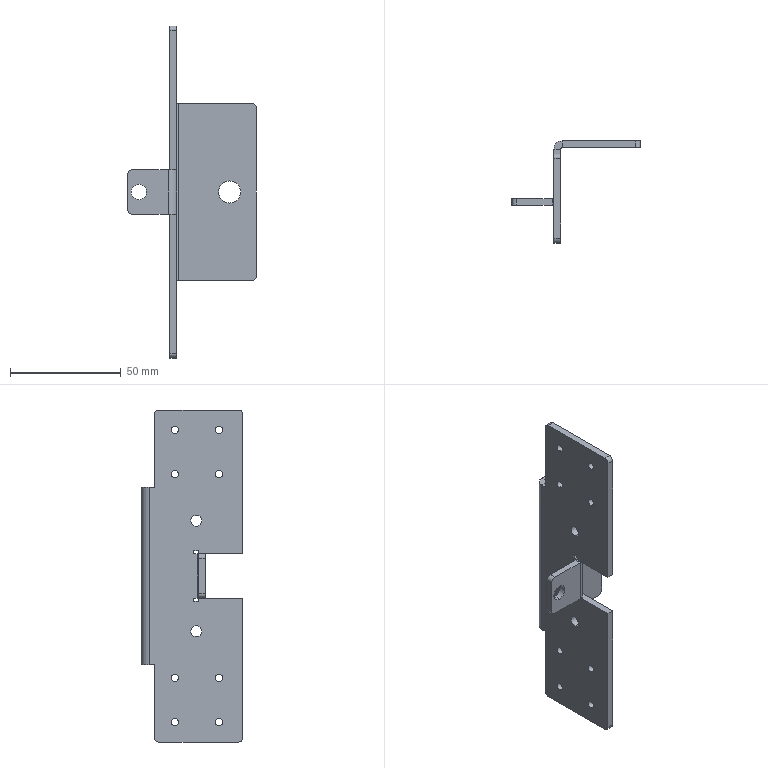Part | NX | features BREP 1 | 1 solid | 70 faces | box 58 x 46 x 150 mm | volume 27197 mm3 | cylinder 36 | plane 34 | commonest cylinder face diameters 3.3 x16 4 x8 5 x4 1.473 x2 7 x2 7.473 x2